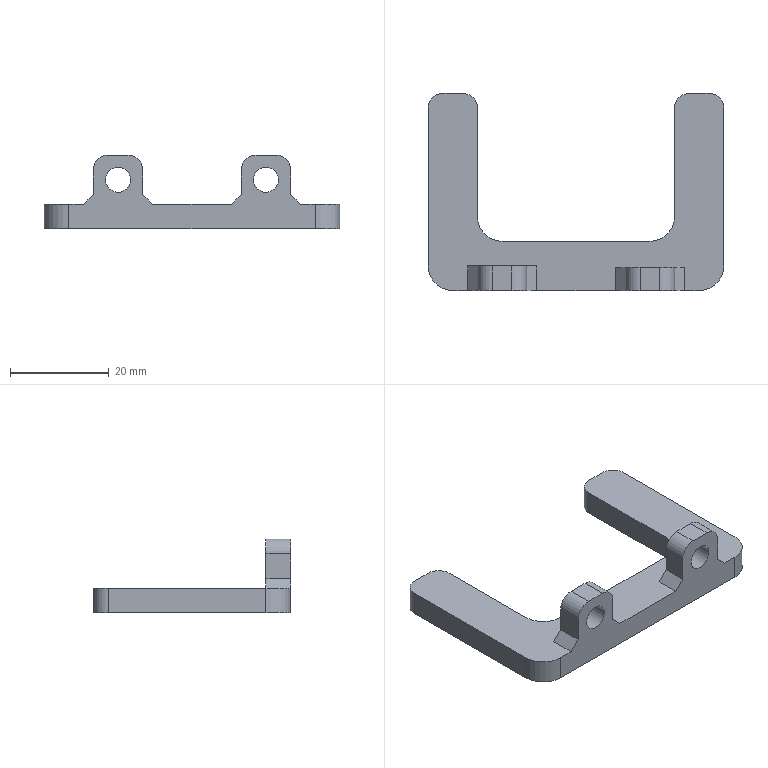Part | NX | features BREP 1 | 1 solid | 36 faces | box 60 x 40 x 15 mm | volume 6735 mm3 | plane 22 | cylinder 14 | commonest cylinder face diameters 6 x8 10 x4 5.1 x2
STEP:
#1=CARTESIAN_POINT('',(15.,-20.,7.45));
#2=VERTEX_POINT('',#1);
#3=CARTESIAN_POINT('',(15.,-20.,10.));
#4=DIRECTION('',(0.,-1.,0.));
#5=DIRECTION('',(0.,0.,-1.));
#6=AXIS2_PLACEMENT_3D('',#3,#4,#5);
#7=CIRCLE('',#6,2.55);
#8=EDGE_CURVE('',#2,#2,#7,.T.);
#9=ORIENTED_EDGE('',*,*,#8,.T.);
#10=EDGE_LOOP('',(#9));
#11=FACE_BOUND('',#10,.T.);
#12=CARTESIAN_POINT('',(15.,-15.3,7.45));
#13=VERTEX_POINT('',#12);
#14=CARTESIAN_POINT('',(15.,-15.3,10.));
#15=DIRECTION('',(0.,-1.,0.));
#16=DIRECTION('',(0.,0.,-1.));
#17=AXIS2_PLACEMENT_3D('',#14,#15,#16);
#18=CIRCLE('',#17,2.55);
#19=EDGE_CURVE('',#13,#13,#18,.T.);
#20=ORIENTED_EDGE('',*,*,#19,.F.);
#21=EDGE_LOOP('',(#20));
#22=FACE_BOUND('',#21,.T.);
#23=CARTESIAN_POINT('',(15.,-10.,10.));
#24=DIRECTION('',(0.,-1.,0.));
#25=DIRECTION('',(0.,0.,1.));
#26=AXIS2_PLACEMENT_3D('',#23,#24,#25);
#27=CYLINDRICAL_SURFACE('',#26,2.55);
#28=ADVANCED_FACE('',(#11,#22),#27,.F.);
#29=CARTESIAN_POINT('',(-15.,-20.,7.45));
#30=VERTEX_POINT('',#29);
#31=CARTESIAN_POINT('',(-15.,-20.,10.));
#32=DIRECTION('',(0.,-1.,0.));
#33=DIRECTION('',(0.,0.,-1.));
#34=AXIS2_PLACEMENT_3D('',#31,#32,#33);
#35=CIRCLE('',#34,2.55);
#36=EDGE_CURVE('',#30,#30,#35,.T.);
#37=ORIENTED_EDGE('',*,*,#36,.T.);
#38=EDGE_LOOP('',(#37));
#39=FACE_BOUND('',#38,.T.);
#40=CARTESIAN_POINT('',(-15.,-15.,7.45));
#41=VERTEX_POINT('',#40);
#42=CARTESIAN_POINT('',(-15.,-15.,10.));
#43=DIRECTION('',(0.,-1.,0.));
#44=DIRECTION('',(0.,0.,-1.));
#45=AXIS2_PLACEMENT_3D('',#42,#43,#44);
#46=CIRCLE('',#45,2.55);
#47=EDGE_CURVE('',#41,#41,#46,.T.);
#48=ORIENTED_EDGE('',*,*,#47,.F.);
#49=EDGE_LOOP('',(#48));
#50=FACE_BOUND('',#49,.T.);
#51=CARTESIAN_POINT('',(-15.,-10.,10.));
#52=DIRECTION('',(0.,-1.,0.));
#53=DIRECTION('',(0.,0.,1.));
#54=AXIS2_PLACEMENT_3D('',#51,#52,#53);
#55=CYLINDRICAL_SURFACE('',#54,2.55);
#56=ADVANCED_FACE('',(#39,#50),#55,.F.);
#57=CARTESIAN_POINT('',(22.,-15.3,5.));
#58=VERTEX_POINT('',#57);
#59=CARTESIAN_POINT('',(8.,-15.3,5.));
#60=VERTEX_POINT('',#59);
#61=CARTESIAN_POINT('',(10.,-15.3,5.));
#62=DIRECTION('',(-1.,0.,0.));
#63=VECTOR('',#62,1000.);
#64=LINE('',#61,#63);
#65=EDGE_CURVE('',#58,#60,#64,.T.);
#66=ORIENTED_EDGE('',*,*,#65,.F.);
#67=CARTESIAN_POINT('',(22.,-20.,5.));
#68=VERTEX_POINT('',#67);
#69=CARTESIAN_POINT('',(22.,0.,5.));
#70=DIRECTION('',(0.,-1.,0.));
#71=VECTOR('',#70,1000.);
#72=LINE('',#69,#71);
#73=EDGE_CURVE('',#58,#68,#72,.T.);
#74=ORIENTED_EDGE('',*,*,#73,.T.);
#75=CARTESIAN_POINT('',(25.,-20.,5.));
#76=VERTEX_POINT('',#75);
#77=CARTESIAN_POINT('',(-30.,-20.,5.));
#78=DIRECTION('',(1.,0.,0.));
#79=VECTOR('',#78,1000.);
#80=LINE('',#77,#79);
#81=EDGE_CURVE('',#68,#76,#80,.T.);
#82=ORIENTED_EDGE('',*,*,#81,.T.);
#83=CARTESIAN_POINT('',(30.,-15.,5.));
#84=VERTEX_POINT('',#83);
#85=CARTESIAN_POINT('',(25.,-15.,5.));
#86=DIRECTION('',(0.,0.,1.));
#87=DIRECTION('',(1.,0.,0.));
#88=AXIS2_PLACEMENT_3D('',#85,#86,#87);
#89=CIRCLE('',#88,5.);
#90=EDGE_CURVE('',#76,#84,#89,.T.);
#91=ORIENTED_EDGE('',*,*,#90,.T.);
#92=CARTESIAN_POINT('',(30.,17.,5.));
#93=VERTEX_POINT('',#92);
#94=CARTESIAN_POINT('',(30.,20.,5.));
#95=DIRECTION('',(0.,1.,0.));
#96=VECTOR('',#95,1000.);
#97=LINE('',#94,#96);
#98=EDGE_CURVE('',#84,#93,#97,.T.);
#99=ORIENTED_EDGE('',*,*,#98,.T.);
#100=CARTESIAN_POINT('',(27.,20.,5.));
#101=VERTEX_POINT('',#100);
#102=CARTESIAN_POINT('',(27.,17.,5.));
#103=DIRECTION('',(0.,0.,1.));
#104=DIRECTION('',(1.,0.,0.));
#105=AXIS2_PLACEMENT_3D('',#102,#103,#104);
#106=CIRCLE('',#105,3.);
#107=EDGE_CURVE('',#93,#101,#106,.T.);
#108=ORIENTED_EDGE('',*,*,#107,.T.);
#109=CARTESIAN_POINT('',(23.,20.,5.));
#110=VERTEX_POINT('',#109);
#111=CARTESIAN_POINT('',(-30.,20.,5.));
#112=DIRECTION('',(-1.,0.,0.));
#113=VECTOR('',#112,1000.);
#114=LINE('',#111,#113);
#115=EDGE_CURVE('',#101,#110,#114,.T.);
#116=ORIENTED_EDGE('',*,*,#115,.T.);
#117=CARTESIAN_POINT('',(20.,17.,5.));
#118=VERTEX_POINT('',#117);
#119=CARTESIAN_POINT('',(23.,17.,5.));
#120=DIRECTION('',(0.,0.,1.));
#121=DIRECTION('',(1.,0.,0.));
#122=AXIS2_PLACEMENT_3D('',#119,#120,#121);
#123=CIRCLE('',#122,3.);
#124=EDGE_CURVE('',#110,#118,#123,.T.);
#125=ORIENTED_EDGE('',*,*,#124,.T.);
#126=CARTESIAN_POINT('',(20.,-5.,5.));
#127=VERTEX_POINT('',#126);
#128=CARTESIAN_POINT('',(20.,20.,5.));
#129=DIRECTION('',(0.,1.,0.));
#130=VECTOR('',#129,1000.);
#131=LINE('',#128,#130);
#132=EDGE_CURVE('',#127,#118,#131,.T.);
#133=ORIENTED_EDGE('',*,*,#132,.F.);
#134=CARTESIAN_POINT('',(15.,-10.,5.));
#135=VERTEX_POINT('',#134);
#136=CARTESIAN_POINT('',(15.,-5.,5.));
#137=DIRECTION('',(0.,0.,-1.));
#138=DIRECTION('',(1.,0.,0.));
#139=AXIS2_PLACEMENT_3D('',#136,#137,#138);
#140=CIRCLE('',#139,5.);
#141=EDGE_CURVE('',#127,#135,#140,.T.);
#142=ORIENTED_EDGE('',*,*,#141,.T.);
#143=CARTESIAN_POINT('',(-15.,-10.,5.));
#144=VERTEX_POINT('',#143);
#145=CARTESIAN_POINT('',(-20.,-10.,5.));
#146=DIRECTION('',(1.,0.,0.));
#147=VECTOR('',#146,1000.);
#148=LINE('',#145,#147);
#149=EDGE_CURVE('',#144,#135,#148,.T.);
#150=ORIENTED_EDGE('',*,*,#149,.F.);
#151=CARTESIAN_POINT('',(-20.,-5.,5.));
#152=VERTEX_POINT('',#151);
#153=CARTESIAN_POINT('',(-15.,-5.,5.));
#154=DIRECTION('',(0.,0.,-1.));
#155=DIRECTION('',(1.,0.,0.));
#156=AXIS2_PLACEMENT_3D('',#153,#154,#155);
#157=CIRCLE('',#156,5.);
#158=EDGE_CURVE('',#144,#152,#157,.T.);
#159=ORIENTED_EDGE('',*,*,#158,.T.);
#160=CARTESIAN_POINT('',(-20.,17.,5.));
#161=VERTEX_POINT('',#160);
#162=CARTESIAN_POINT('',(-20.,20.,5.));
#163=DIRECTION('',(0.,-1.,0.));
#164=VECTOR('',#163,1000.);
#165=LINE('',#162,#164);
#166=EDGE_CURVE('',#161,#152,#165,.T.);
#167=ORIENTED_EDGE('',*,*,#166,.F.);
#168=CARTESIAN_POINT('',(-23.,20.,5.));
#169=VERTEX_POINT('',#168);
#170=CARTESIAN_POINT('',(-23.,17.,5.));
#171=DIRECTION('',(0.,0.,1.));
#172=DIRECTION('',(1.,0.,0.));
#173=AXIS2_PLACEMENT_3D('',#170,#171,#172);
#174=CIRCLE('',#173,3.);
#175=EDGE_CURVE('',#161,#169,#174,.T.);
#176=ORIENTED_EDGE('',*,*,#175,.T.);
#177=CARTESIAN_POINT('',(-27.,20.,5.));
#178=VERTEX_POINT('',#177);
#179=CARTESIAN_POINT('',(-30.,20.,5.));
#180=DIRECTION('',(-1.,0.,0.));
#181=VECTOR('',#180,1000.);
#182=LINE('',#179,#181);
#183=EDGE_CURVE('',#169,#178,#182,.T.);
#184=ORIENTED_EDGE('',*,*,#183,.T.);
#185=CARTESIAN_POINT('',(-30.,17.,5.));
#186=VERTEX_POINT('',#185);
#187=CARTESIAN_POINT('',(-27.,17.,5.));
#188=DIRECTION('',(0.,0.,1.));
#189=DIRECTION('',(1.,0.,0.));
#190=AXIS2_PLACEMENT_3D('',#187,#188,#189);
#191=CIRCLE('',#190,3.);
#192=EDGE_CURVE('',#178,#186,#191,.T.);
#193=ORIENTED_EDGE('',*,*,#192,.T.);
#194=CARTESIAN_POINT('',(-30.,-15.,5.));
#195=VERTEX_POINT('',#194);
#196=CARTESIAN_POINT('',(-30.,20.,5.));
#197=DIRECTION('',(0.,-1.,0.));
#198=VECTOR('',#197,1000.);
#199=LINE('',#196,#198);
#200=EDGE_CURVE('',#186,#195,#199,.T.);
#201=ORIENTED_EDGE('',*,*,#200,.T.);
#202=CARTESIAN_POINT('',(-25.,-20.,5.));
#203=VERTEX_POINT('',#202);
#204=CARTESIAN_POINT('',(-25.,-15.,5.));
#205=DIRECTION('',(0.,0.,1.));
#206=DIRECTION('',(1.,0.,0.));
#207=AXIS2_PLACEMENT_3D('',#204,#205,#206);
#208=CIRCLE('',#207,5.);
#209=EDGE_CURVE('',#195,#203,#208,.T.);
#210=ORIENTED_EDGE('',*,*,#209,.T.);
#211=CARTESIAN_POINT('',(-22.,-20.,5.));
#212=VERTEX_POINT('',#211);
#213=CARTESIAN_POINT('',(-30.,-20.,5.));
#214=DIRECTION('',(1.,0.,0.));
#215=VECTOR('',#214,1000.);
#216=LINE('',#213,#215);
#217=EDGE_CURVE('',#203,#212,#216,.T.);
#218=ORIENTED_EDGE('',*,*,#217,.T.);
#219=CARTESIAN_POINT('',(-22.,-15.,5.));
#220=VERTEX_POINT('',#219);
#221=CARTESIAN_POINT('',(-22.,0.,5.));
#222=DIRECTION('',(0.,1.,0.));
#223=VECTOR('',#222,1000.);
#224=LINE('',#221,#223);
#225=EDGE_CURVE('',#212,#220,#224,.T.);
#226=ORIENTED_EDGE('',*,*,#225,.T.);
#227=CARTESIAN_POINT('',(-8.,-15.,5.));
#228=VERTEX_POINT('',#227);
#229=CARTESIAN_POINT('',(-20.,-15.,5.));
#230=DIRECTION('',(-1.,0.,0.));
#231=VECTOR('',#230,1000.);
#232=LINE('',#229,#231);
#233=EDGE_CURVE('',#228,#220,#232,.T.);
#234=ORIENTED_EDGE('',*,*,#233,.F.);
#235=CARTESIAN_POINT('',(-8.,-20.,5.));
#236=VERTEX_POINT('',#235);
#237=CARTESIAN_POINT('',(-8.,0.,5.));
#238=DIRECTION('',(0.,-1.,0.));
#239=VECTOR('',#238,1000.);
#240=LINE('',#237,#239);
#241=EDGE_CURVE('',#228,#236,#240,.T.);
#242=ORIENTED_EDGE('',*,*,#241,.T.);
#243=CARTESIAN_POINT('',(8.,-20.,5.));
#244=VERTEX_POINT('',#243);
#245=CARTESIAN_POINT('',(-30.,-20.,5.));
#246=DIRECTION('',(1.,0.,0.));
#247=VECTOR('',#246,1000.);
#248=LINE('',#245,#247);
#249=EDGE_CURVE('',#236,#244,#248,.T.);
#250=ORIENTED_EDGE('',*,*,#249,.T.);
#251=CARTESIAN_POINT('',(8.,0.,5.));
#252=DIRECTION('',(0.,1.,0.));
#253=VECTOR('',#252,1000.);
#254=LINE('',#251,#253);
#255=EDGE_CURVE('',#244,#60,#254,.T.);
#256=ORIENTED_EDGE('',*,*,#255,.T.);
#257=EDGE_LOOP('',(#66,#74,#82,#91,#99,#108,#116,#125,#133,#142,#150,#159,#167,#176,#184,#193,#201,#210,#218,#226,#234,#242,#250,#256));
#258=FACE_BOUND('',#257,.T.);
#259=CARTESIAN_POINT('',(0.,0.,5.));
#260=DIRECTION('',(0.,0.,1.));
#261=DIRECTION('',(-1.,0.,0.));
#262=AXIS2_PLACEMENT_3D('',#259,#260,#261);
#263=PLANE('',#262);
#264=ADVANCED_FACE('',(#258),#263,.T.);
#265=CARTESIAN_POINT('',(-23.,20.,0.));
#266=VERTEX_POINT('',#265);
#267=CARTESIAN_POINT('',(-27.,20.,0.));
#268=VERTEX_POINT('',#267);
#269=CARTESIAN_POINT('',(-30.,20.,0.));
#270=DIRECTION('',(-1.,0.,0.));
#271=VECTOR('',#270,1000.);
#272=LINE('',#269,#271);
#273=EDGE_CURVE('',#266,#268,#272,.T.);
#274=ORIENTED_EDGE('',*,*,#273,.T.);
#275=CARTESIAN_POINT('',(-27.,20.,5.));
#276=DIRECTION('',(0.,0.,1.));
#277=VECTOR('',#276,1000.);
#278=LINE('',#275,#277);
#279=EDGE_CURVE('',#268,#178,#278,.T.);
#280=ORIENTED_EDGE('',*,*,#279,.T.);
#281=ORIENTED_EDGE('',*,*,#183,.F.);
#282=CARTESIAN_POINT('',(-23.,20.,5.));
#283=DIRECTION('',(0.,0.,-1.));
#284=VECTOR('',#283,1000.);
#285=LINE('',#282,#284);
#286=EDGE_CURVE('',#169,#266,#285,.T.);
#287=ORIENTED_EDGE('',*,*,#286,.T.);
#288=EDGE_LOOP('',(#274,#280,#281,#287));
#289=FACE_BOUND('',#288,.T.);
#290=CARTESIAN_POINT('',(-30.,20.,5.));
#291=DIRECTION('',(0.,-1.,0.));
#292=DIRECTION('',(0.,0.,1.));
#293=AXIS2_PLACEMENT_3D('',#290,#291,#292);
#294=PLANE('',#293);
#295=ADVANCED_FACE('',(#289),#294,.F.);
#296=CARTESIAN_POINT('',(30.,-15.,0.));
#297=VERTEX_POINT('',#296);
#298=CARTESIAN_POINT('',(30.,17.,0.));
#299=VERTEX_POINT('',#298);
#300=CARTESIAN_POINT('',(30.,20.,0.));
#301=DIRECTION('',(0.,1.,0.));
#302=VECTOR('',#301,1000.);
#303=LINE('',#300,#302);
#304=EDGE_CURVE('',#297,#299,#303,.T.);
#305=ORIENTED_EDGE('',*,*,#304,.T.);
#306=CARTESIAN_POINT('',(30.,17.,5.));
#307=DIRECTION('',(0.,0.,1.));
#308=VECTOR('',#307,1000.);
#309=LINE('',#306,#308);
#310=EDGE_CURVE('',#299,#93,#309,.T.);
#311=ORIENTED_EDGE('',*,*,#310,.T.);
#312=ORIENTED_EDGE('',*,*,#98,.F.);
#313=CARTESIAN_POINT('',(30.,-15.,5.));
#314=DIRECTION('',(0.,0.,-1.));
#315=VECTOR('',#314,1000.);
#316=LINE('',#313,#315);
#317=EDGE_CURVE('',#84,#297,#316,.T.);
#318=ORIENTED_EDGE('',*,*,#317,.T.);
#319=EDGE_LOOP('',(#305,#311,#312,#318));
#320=FACE_BOUND('',#319,.T.);
#321=CARTESIAN_POINT('',(30.,20.,5.));
#322=DIRECTION('',(-1.,0.,0.));
#323=DIRECTION('',(0.,1.,0.));
#324=AXIS2_PLACEMENT_3D('',#321,#322,#323);
#325=PLANE('',#324);
#326=ADVANCED_FACE('',(#320),#325,.F.);
#327=ORIENTED_EDGE('',*,*,#115,.F.);
#328=CARTESIAN_POINT('',(27.,20.,0.));
#329=VERTEX_POINT('',#328);
#330=CARTESIAN_POINT('',(27.,20.,5.));
#331=DIRECTION('',(0.,0.,-1.));
#332=VECTOR('',#331,1000.);
#333=LINE('',#330,#332);
#334=EDGE_CURVE('',#101,#329,#333,.T.);
#335=ORIENTED_EDGE('',*,*,#334,.T.);
#336=CARTESIAN_POINT('',(23.,20.,0.));
#337=VERTEX_POINT('',#336);
#338=CARTESIAN_POINT('',(-30.,20.,0.));
#339=DIRECTION('',(-1.,0.,0.));
#340=VECTOR('',#339,1000.);
#341=LINE('',#338,#340);
#342=EDGE_CURVE('',#329,#337,#341,.T.);
#343=ORIENTED_EDGE('',*,*,#342,.T.);
#344=CARTESIAN_POINT('',(23.,20.,5.));
#345=DIRECTION('',(0.,0.,1.));
#346=VECTOR('',#345,1000.);
#347=LINE('',#344,#346);
#348=EDGE_CURVE('',#337,#110,#347,.T.);
#349=ORIENTED_EDGE('',*,*,#348,.T.);
#350=EDGE_LOOP('',(#327,#335,#343,#349));
#351=FACE_BOUND('',#350,.T.);
#352=CARTESIAN_POINT('',(-30.,20.,5.));
#353=DIRECTION('',(0.,-1.,0.));
#354=DIRECTION('',(0.,0.,1.));
#355=AXIS2_PLACEMENT_3D('',#352,#353,#354);
#356=PLANE('',#355);
#357=ADVANCED_FACE('',(#351),#356,.F.);
#358=ORIENTED_EDGE('',*,*,#200,.F.);
#359=CARTESIAN_POINT('',(-30.,17.,0.));
#360=VERTEX_POINT('',#359);
#361=CARTESIAN_POINT('',(-30.,17.,5.));
#362=DIRECTION('',(0.,0.,-1.));
#363=VECTOR('',#362,1000.);
#364=LINE('',#361,#363);
#365=EDGE_CURVE('',#186,#360,#364,.T.);
#366=ORIENTED_EDGE('',*,*,#365,.T.);
#367=CARTESIAN_POINT('',(-30.,-15.,0.));
#368=VERTEX_POINT('',#367);
#369=CARTESIAN_POINT('',(-30.,20.,0.));
#370=DIRECTION('',(0.,-1.,0.));
#371=VECTOR('',#370,1000.);
#372=LINE('',#369,#371);
#373=EDGE_CURVE('',#360,#368,#372,.T.);
#374=ORIENTED_EDGE('',*,*,#373,.T.);
#375=CARTESIAN_POINT('',(-30.,-15.,5.));
#376=DIRECTION('',(0.,0.,1.));
#377=VECTOR('',#376,1000.);
#378=LINE('',#375,#377);
#379=EDGE_CURVE('',#368,#195,#378,.T.);
#380=ORIENTED_EDGE('',*,*,#379,.T.);
#381=EDGE_LOOP('',(#358,#366,#374,#380));
#382=FACE_BOUND('',#381,.T.);
#383=CARTESIAN_POINT('',(-30.,20.,5.));
#384=DIRECTION('',(1.,0.,0.));
#385=DIRECTION('',(0.,-1.,0.));
#386=AXIS2_PLACEMENT_3D('',#383,#384,#385);
#387=PLANE('',#386);
#388=ADVANCED_FACE('',(#382),#387,.F.);
#389=ORIENTED_EDGE('',*,*,#8,.F.);
#390=EDGE_LOOP('',(#389));
#391=FACE_BOUND('',#390,.T.);
#392=ORIENTED_EDGE('',*,*,#36,.F.);
#393=EDGE_LOOP('',(#392));
#394=FACE_BOUND('',#393,.T.);
#395=CARTESIAN_POINT('',(-17.,-20.,15.));
#396=VERTEX_POINT('',#395);
#397=CARTESIAN_POINT('',(-13.,-20.,15.));
#398=VERTEX_POINT('',#397);
#399=CARTESIAN_POINT('',(-20.,-20.,15.));
#400=DIRECTION('',(1.,0.,0.));
#401=VECTOR('',#400,1000.);
#402=LINE('',#399,#401);
#403=EDGE_CURVE('',#396,#398,#402,.T.);
#404=ORIENTED_EDGE('',*,*,#403,.F.);
#405=CARTESIAN_POINT('',(-20.,-20.,12.));
#406=VERTEX_POINT('',#405);
#407=CARTESIAN_POINT('',(-17.,-20.,12.));
#408=DIRECTION('',(0.,-1.,0.));
#409=DIRECTION('',(0.,0.,1.));
#410=AXIS2_PLACEMENT_3D('',#407,#408,#409);
#411=CIRCLE('',#410,3.);
#412=EDGE_CURVE('',#396,#406,#411,.T.);
#413=ORIENTED_EDGE('',*,*,#412,.T.);
#414=CARTESIAN_POINT('',(-20.,-20.,7.));
#415=VERTEX_POINT('',#414);
#416=CARTESIAN_POINT('',(-20.,-20.,15.));
#417=DIRECTION('',(0.,0.,-1.));
#418=VECTOR('',#417,1000.);
#419=LINE('',#416,#418);
#420=EDGE_CURVE('',#406,#415,#419,.T.);
#421=ORIENTED_EDGE('',*,*,#420,.T.);
#422=CARTESIAN_POINT('',(-26.,-20.,1.));
#423=DIRECTION('',(-0.7071,0.,-0.7071));
#424=VECTOR('',#423,1000.);
#425=LINE('',#422,#424);
#426=EDGE_CURVE('',#415,#212,#425,.T.);
#427=ORIENTED_EDGE('',*,*,#426,.T.);
#428=ORIENTED_EDGE('',*,*,#217,.F.);
#429=CARTESIAN_POINT('',(-25.,-20.,0.));
#430=VERTEX_POINT('',#429);
#431=CARTESIAN_POINT('',(-25.,-20.,5.));
#432=DIRECTION('',(0.,0.,-1.));
#433=VECTOR('',#432,1000.);
#434=LINE('',#431,#433);
#435=EDGE_CURVE('',#203,#430,#434,.T.);
#436=ORIENTED_EDGE('',*,*,#435,.T.);
#437=CARTESIAN_POINT('',(25.,-20.,0.));
#438=VERTEX_POINT('',#437);
#439=CARTESIAN_POINT('',(-30.,-20.,0.));
#440=DIRECTION('',(1.,0.,0.));
#441=VECTOR('',#440,1000.);
#442=LINE('',#439,#441);
#443=EDGE_CURVE('',#430,#438,#442,.T.);
#444=ORIENTED_EDGE('',*,*,#443,.T.);
#445=CARTESIAN_POINT('',(25.,-20.,5.));
#446=DIRECTION('',(0.,0.,1.));
#447=VECTOR('',#446,1000.);
#448=LINE('',#445,#447);
#449=EDGE_CURVE('',#438,#76,#448,.T.);
#450=ORIENTED_EDGE('',*,*,#449,.T.);
#451=ORIENTED_EDGE('',*,*,#81,.F.);
#452=CARTESIAN_POINT('',(20.,-20.,7.));
#453=VERTEX_POINT('',#452);
#454=CARTESIAN_POINT('',(-4.,-20.,31.));
#455=DIRECTION('',(-0.7071,0.,0.7071));
#456=VECTOR('',#455,1000.);
#457=LINE('',#454,#456);
#458=EDGE_CURVE('',#68,#453,#457,.T.);
#459=ORIENTED_EDGE('',*,*,#458,.T.);
#460=CARTESIAN_POINT('',(20.,-20.,12.));
#461=VERTEX_POINT('',#460);
#462=CARTESIAN_POINT('',(20.,-20.,15.));
#463=DIRECTION('',(0.,0.,-1.));
#464=VECTOR('',#463,1000.);
#465=LINE('',#462,#464);
#466=EDGE_CURVE('',#461,#453,#465,.T.);
#467=ORIENTED_EDGE('',*,*,#466,.F.);
#468=CARTESIAN_POINT('',(17.,-20.,15.));
#469=VERTEX_POINT('',#468);
#470=CARTESIAN_POINT('',(17.,-20.,12.));
#471=DIRECTION('',(0.,-1.,0.));
#472=DIRECTION('',(0.,0.,1.));
#473=AXIS2_PLACEMENT_3D('',#470,#471,#472);
#474=CIRCLE('',#473,3.);
#475=EDGE_CURVE('',#461,#469,#474,.T.);
#476=ORIENTED_EDGE('',*,*,#475,.T.);
#477=CARTESIAN_POINT('',(13.,-20.,15.));
#478=VERTEX_POINT('',#477);
#479=CARTESIAN_POINT('',(10.,-20.,15.));
#480=DIRECTION('',(1.,0.,0.));
#481=VECTOR('',#480,1000.);
#482=LINE('',#479,#481);
#483=EDGE_CURVE('',#478,#469,#482,.T.);
#484=ORIENTED_EDGE('',*,*,#483,.F.);
#485=CARTESIAN_POINT('',(10.,-20.,12.));
#486=VERTEX_POINT('',#485);
#487=CARTESIAN_POINT('',(13.,-20.,12.));
#488=DIRECTION('',(0.,-1.,0.));
#489=DIRECTION('',(0.,0.,1.));
#490=AXIS2_PLACEMENT_3D('',#487,#488,#489);
#491=CIRCLE('',#490,3.);
#492=EDGE_CURVE('',#478,#486,#491,.T.);
#493=ORIENTED_EDGE('',*,*,#492,.T.);
#494=CARTESIAN_POINT('',(10.,-20.,7.));
#495=VERTEX_POINT('',#494);
#496=CARTESIAN_POINT('',(10.,-20.,15.));
#497=DIRECTION('',(0.,0.,-1.));
#498=VECTOR('',#497,1000.);
#499=LINE('',#496,#498);
#500=EDGE_CURVE('',#486,#495,#499,.T.);
#501=ORIENTED_EDGE('',*,*,#500,.T.);
#502=CARTESIAN_POINT('',(-11.,-20.,-14.));
#503=DIRECTION('',(-0.7071,0.,-0.7071));
#504=VECTOR('',#503,1000.);
#505=LINE('',#502,#504);
#506=EDGE_CURVE('',#495,#244,#505,.T.);
#507=ORIENTED_EDGE('',*,*,#506,.T.);
#508=ORIENTED_EDGE('',*,*,#249,.F.);
#509=CARTESIAN_POINT('',(-10.,-20.,7.));
#510=VERTEX_POINT('',#509);
#511=CARTESIAN_POINT('',(-19.,-20.,16.));
#512=DIRECTION('',(-0.7071,0.,0.7071));
#513=VECTOR('',#512,1000.);
#514=LINE('',#511,#513);
#515=EDGE_CURVE('',#236,#510,#514,.T.);
#516=ORIENTED_EDGE('',*,*,#515,.T.);
#517=CARTESIAN_POINT('',(-10.,-20.,12.));
#518=VERTEX_POINT('',#517);
#519=CARTESIAN_POINT('',(-10.,-20.,15.));
#520=DIRECTION('',(0.,0.,-1.));
#521=VECTOR('',#520,1000.);
#522=LINE('',#519,#521);
#523=EDGE_CURVE('',#518,#510,#522,.T.);
#524=ORIENTED_EDGE('',*,*,#523,.F.);
#525=CARTESIAN_POINT('',(-13.,-20.,12.));
#526=DIRECTION('',(0.,-1.,0.));
#527=DIRECTION('',(0.,0.,1.));
#528=AXIS2_PLACEMENT_3D('',#525,#526,#527);
#529=CIRCLE('',#528,3.);
#530=EDGE_CURVE('',#518,#398,#529,.T.);
#531=ORIENTED_EDGE('',*,*,#530,.T.);
#532=EDGE_LOOP('',(#404,#413,#421,#427,#428,#436,#444,#450,#451,#459,#467,#476,#484,#493,#501,#507,#508,#516,#524,#531));
#533=FACE_BOUND('',#532,.T.);
#534=CARTESIAN_POINT('',(-30.,-20.,5.));
#535=DIRECTION('',(0.,1.,0.));
#536=DIRECTION('',(0.,0.,-1.));
#537=AXIS2_PLACEMENT_3D('',#534,#535,#536);
#538=PLANE('',#537);
#539=ADVANCED_FACE('',(#391,#394,#533),#538,.F.);
#540=ORIENTED_EDGE('',*,*,#342,.F.);
#541=CARTESIAN_POINT('',(27.,17.,0.));
#542=DIRECTION('',(0.,0.,-1.));
#543=DIRECTION('',(1.,0.,0.));
#544=AXIS2_PLACEMENT_3D('',#541,#542,#543);
#545=CIRCLE('',#544,3.);
#546=EDGE_CURVE('',#329,#299,#545,.T.);
#547=ORIENTED_EDGE('',*,*,#546,.T.);
#548=ORIENTED_EDGE('',*,*,#304,.F.);
#549=CARTESIAN_POINT('',(25.,-15.,0.));
#550=DIRECTION('',(0.,0.,-1.));
#551=DIRECTION('',(1.,0.,0.));
#552=AXIS2_PLACEMENT_3D('',#549,#550,#551);
#553=CIRCLE('',#552,5.);
#554=EDGE_CURVE('',#297,#438,#553,.T.);
#555=ORIENTED_EDGE('',*,*,#554,.T.);
#556=ORIENTED_EDGE('',*,*,#443,.F.);
#557=CARTESIAN_POINT('',(-25.,-15.,0.));
#558=DIRECTION('',(0.,0.,-1.));
#559=DIRECTION('',(1.,0.,0.));
#560=AXIS2_PLACEMENT_3D('',#557,#558,#559);
#561=CIRCLE('',#560,5.);
#562=EDGE_CURVE('',#430,#368,#561,.T.);
#563=ORIENTED_EDGE('',*,*,#562,.T.);
#564=ORIENTED_EDGE('',*,*,#373,.F.);
#565=CARTESIAN_POINT('',(-27.,17.,0.));
#566=DIRECTION('',(0.,0.,-1.));
#567=DIRECTION('',(1.,0.,0.));
#568=AXIS2_PLACEMENT_3D('',#565,#566,#567);
#569=CIRCLE('',#568,3.);
#570=EDGE_CURVE('',#360,#268,#569,.T.);
#571=ORIENTED_EDGE('',*,*,#570,.T.);
#572=ORIENTED_EDGE('',*,*,#273,.F.);
#573=CARTESIAN_POINT('',(-20.,17.,0.));
#574=VERTEX_POINT('',#573);
#575=CARTESIAN_POINT('',(-23.,17.,0.));
#576=DIRECTION('',(0.,0.,-1.));
#577=DIRECTION('',(1.,0.,0.));
#578=AXIS2_PLACEMENT_3D('',#575,#576,#577);
#579=CIRCLE('',#578,3.);
#580=EDGE_CURVE('',#266,#574,#579,.T.);
#581=ORIENTED_EDGE('',*,*,#580,.T.);
#582=CARTESIAN_POINT('',(-20.,-5.,0.));
#583=VERTEX_POINT('',#582);
#584=CARTESIAN_POINT('',(-20.,20.,0.));
#585=DIRECTION('',(0.,-1.,0.));
#586=VECTOR('',#585,1000.);
#587=LINE('',#584,#586);
#588=EDGE_CURVE('',#574,#583,#587,.T.);
#589=ORIENTED_EDGE('',*,*,#588,.T.);
#590=CARTESIAN_POINT('',(-15.,-10.,0.));
#591=VERTEX_POINT('',#590);
#592=CARTESIAN_POINT('',(-15.,-5.,0.));
#593=DIRECTION('',(0.,0.,1.));
#594=DIRECTION('',(1.,0.,0.));
#595=AXIS2_PLACEMENT_3D('',#592,#593,#594);
#596=CIRCLE('',#595,5.);
#597=EDGE_CURVE('',#583,#591,#596,.T.);
#598=ORIENTED_EDGE('',*,*,#597,.T.);
#599=CARTESIAN_POINT('',(15.,-10.,0.));
#600=VERTEX_POINT('',#599);
#601=CARTESIAN_POINT('',(-20.,-10.,0.));
#602=DIRECTION('',(1.,0.,0.));
#603=VECTOR('',#602,1000.);
#604=LINE('',#601,#603);
#605=EDGE_CURVE('',#591,#600,#604,.T.);
#606=ORIENTED_EDGE('',*,*,#605,.T.);
#607=CARTESIAN_POINT('',(20.,-5.,0.));
#608=VERTEX_POINT('',#607);
#609=CARTESIAN_POINT('',(15.,-5.,0.));
#610=DIRECTION('',(0.,0.,1.));
#611=DIRECTION('',(1.,0.,0.));
#612=AXIS2_PLACEMENT_3D('',#609,#610,#611);
#613=CIRCLE('',#612,5.);
#614=EDGE_CURVE('',#600,#608,#613,.T.);
#615=ORIENTED_EDGE('',*,*,#614,.T.);
#616=CARTESIAN_POINT('',(20.,17.,0.));
#617=VERTEX_POINT('',#616);
#618=CARTESIAN_POINT('',(20.,20.,0.));
#619=DIRECTION('',(0.,1.,0.));
#620=VECTOR('',#619,1000.);
#621=LINE('',#618,#620);
#622=EDGE_CURVE('',#608,#617,#621,.T.);
#623=ORIENTED_EDGE('',*,*,#622,.T.);
#624=CARTESIAN_POINT('',(23.,17.,0.));
#625=DIRECTION('',(0.,0.,-1.));
#626=DIRECTION('',(1.,0.,0.));
#627=AXIS2_PLACEMENT_3D('',#624,#625,#626);
#628=CIRCLE('',#627,3.);
#629=EDGE_CURVE('',#617,#337,#628,.T.);
#630=ORIENTED_EDGE('',*,*,#629,.T.);
#631=EDGE_LOOP('',(#540,#547,#548,#555,#556,#563,#564,#571,#572,#581,#589,#598,#606,#615,#623,#630));
#632=FACE_BOUND('',#631,.T.);
#633=CARTESIAN_POINT('',(0.,0.,0.));
#634=DIRECTION('',(0.,0.,1.));
#635=DIRECTION('',(-1.,0.,0.));
#636=AXIS2_PLACEMENT_3D('',#633,#634,#635);
#637=PLANE('',#636);
#638=ADVANCED_FACE('',(#632),#637,.F.);
#639=ORIENTED_EDGE('',*,*,#588,.F.);
#640=CARTESIAN_POINT('',(-20.,17.,0.));
#641=DIRECTION('',(0.,0.,1.));
#642=VECTOR('',#641,1000.);
#643=LINE('',#640,#642);
#644=EDGE_CURVE('',#574,#161,#643,.T.);
#645=ORIENTED_EDGE('',*,*,#644,.T.);
#646=ORIENTED_EDGE('',*,*,#166,.T.);
#647=CARTESIAN_POINT('',(-20.,-5.,0.));
#648=DIRECTION('',(0.,0.,-1.));
#649=VECTOR('',#648,1000.);
#650=LINE('',#647,#649);
#651=EDGE_CURVE('',#152,#583,#650,.T.);
#652=ORIENTED_EDGE('',*,*,#651,.T.);
#653=EDGE_LOOP('',(#639,#645,#646,#652));
#654=FACE_BOUND('',#653,.T.);
#655=CARTESIAN_POINT('',(-20.,20.,0.));
#656=DIRECTION('',(-1.,0.,0.));
#657=DIRECTION('',(0.,1.,0.));
#658=AXIS2_PLACEMENT_3D('',#655,#656,#657);
#659=PLANE('',#658);
#660=ADVANCED_FACE('',(#654),#659,.F.);
#661=ORIENTED_EDGE('',*,*,#132,.T.);
#662=CARTESIAN_POINT('',(20.,17.,0.));
#663=DIRECTION('',(0.,0.,-1.));
#664=VECTOR('',#663,1000.);
#665=LINE('',#662,#664);
#666=EDGE_CURVE('',#118,#617,#665,.T.);
#667=ORIENTED_EDGE('',*,*,#666,.T.);
#668=ORIENTED_EDGE('',*,*,#622,.F.);
#669=CARTESIAN_POINT('',(20.,-5.,5.));
#670=DIRECTION('',(0.,0.,1.));
#671=VECTOR('',#670,1000.);
#672=LINE('',#669,#671);
#673=EDGE_CURVE('',#608,#127,#672,.T.);
#674=ORIENTED_EDGE('',*,*,#673,.T.);
#675=EDGE_LOOP('',(#661,#667,#668,#674));
#676=FACE_BOUND('',#675,.T.);
#677=CARTESIAN_POINT('',(20.,20.,0.));
#678=DIRECTION('',(1.,0.,0.));
#679=DIRECTION('',(0.,-1.,0.));
#680=AXIS2_PLACEMENT_3D('',#677,#678,#679);
#681=PLANE('',#680);
#682=ADVANCED_FACE('',(#676),#681,.F.);
#683=ORIENTED_EDGE('',*,*,#149,.T.);
#684=CARTESIAN_POINT('',(15.,-10.,0.));
#685=DIRECTION('',(0.,0.,-1.));
#686=VECTOR('',#685,1000.);
#687=LINE('',#684,#686);
#688=EDGE_CURVE('',#135,#600,#687,.T.);
#689=ORIENTED_EDGE('',*,*,#688,.T.);
#690=ORIENTED_EDGE('',*,*,#605,.F.);
#691=CARTESIAN_POINT('',(-15.,-10.,5.));
#692=DIRECTION('',(0.,0.,1.));
#693=VECTOR('',#692,1000.);
#694=LINE('',#691,#693);
#695=EDGE_CURVE('',#591,#144,#694,.T.);
#696=ORIENTED_EDGE('',*,*,#695,.T.);
#697=EDGE_LOOP('',(#683,#689,#690,#696));
#698=FACE_BOUND('',#697,.T.);
#699=CARTESIAN_POINT('',(-20.,-10.,0.));
#700=DIRECTION('',(0.,-1.,0.));
#701=DIRECTION('',(0.,0.,1.));
#702=AXIS2_PLACEMENT_3D('',#699,#700,#701);
#703=PLANE('',#702);
#704=ADVANCED_FACE('',(#698),#703,.F.);
#705=CARTESIAN_POINT('',(-20.,-15.,12.));
#706=VERTEX_POINT('',#705);
#707=CARTESIAN_POINT('',(-20.,-15.,7.));
#708=VERTEX_POINT('',#707);
#709=CARTESIAN_POINT('',(-20.,-15.,15.));
#710=DIRECTION('',(0.,0.,-1.));
#711=VECTOR('',#710,1000.);
#712=LINE('',#709,#711);
#713=EDGE_CURVE('',#706,#708,#712,.T.);
#714=ORIENTED_EDGE('',*,*,#713,.T.);
#715=CARTESIAN_POINT('',(-20.,-20.,7.));
#716=DIRECTION('',(0.,-1.,0.));
#717=VECTOR('',#716,1000.);
#718=LINE('',#715,#717);
#719=EDGE_CURVE('',#708,#415,#718,.T.);
#720=ORIENTED_EDGE('',*,*,#719,.T.);
#721=ORIENTED_EDGE('',*,*,#420,.F.);
#722=CARTESIAN_POINT('',(-20.,-20.,12.));
#723=DIRECTION('',(0.,1.,0.));
#724=VECTOR('',#723,1000.);
#725=LINE('',#722,#724);
#726=EDGE_CURVE('',#406,#706,#725,.T.);
#727=ORIENTED_EDGE('',*,*,#726,.T.);
#728=EDGE_LOOP('',(#714,#720,#721,#727));
#729=FACE_BOUND('',#728,.T.);
#730=CARTESIAN_POINT('',(-20.,-20.,15.));
#731=DIRECTION('',(1.,0.,0.));
#732=DIRECTION('',(0.,0.,1.));
#733=AXIS2_PLACEMENT_3D('',#730,#731,#732);
#734=PLANE('',#733);
#735=ADVANCED_FACE('',(#729),#734,.F.);
#736=ORIENTED_EDGE('',*,*,#523,.T.);
#737=CARTESIAN_POINT('',(-10.,-15.,7.));
#738=VERTEX_POINT('',#737);
#739=CARTESIAN_POINT('',(-10.,-20.,7.));
#740=DIRECTION('',(0.,1.,0.));
#741=VECTOR('',#740,1000.);
#742=LINE('',#739,#741);
#743=EDGE_CURVE('',#510,#738,#742,.T.);
#744=ORIENTED_EDGE('',*,*,#743,.T.);
#745=CARTESIAN_POINT('',(-10.,-15.,12.));
#746=VERTEX_POINT('',#745);
#747=CARTESIAN_POINT('',(-10.,-15.,15.));
#748=DIRECTION('',(0.,0.,-1.));
#749=VECTOR('',#748,1000.);
#750=LINE('',#747,#749);
#751=EDGE_CURVE('',#746,#738,#750,.T.);
#752=ORIENTED_EDGE('',*,*,#751,.F.);
#753=CARTESIAN_POINT('',(-10.,-20.,12.));
#754=DIRECTION('',(0.,-1.,0.));
#755=VECTOR('',#754,1000.);
#756=LINE('',#753,#755);
#757=EDGE_CURVE('',#746,#518,#756,.T.);
#758=ORIENTED_EDGE('',*,*,#757,.T.);
#759=EDGE_LOOP('',(#736,#744,#752,#758));
#760=FACE_BOUND('',#759,.T.);
#761=CARTESIAN_POINT('',(-10.,-20.,15.));
#762=DIRECTION('',(-1.,0.,0.));
#763=DIRECTION('',(0.,0.,-1.));
#764=AXIS2_PLACEMENT_3D('',#761,#762,#763);
#765=PLANE('',#764);
#766=ADVANCED_FACE('',(#760),#765,.F.);
#767=ORIENTED_EDGE('',*,*,#47,.T.);
#768=EDGE_LOOP('',(#767));
#769=FACE_BOUND('',#768,.T.);
#770=ORIENTED_EDGE('',*,*,#713,.F.);
#771=CARTESIAN_POINT('',(-17.,-15.,15.));
#772=VERTEX_POINT('',#771);
#773=CARTESIAN_POINT('',(-17.,-15.,12.));
#774=DIRECTION('',(0.,1.,0.));
#775=DIRECTION('',(0.,0.,-1.));
#776=AXIS2_PLACEMENT_3D('',#773,#774,#775);
#777=CIRCLE('',#776,3.);
#778=EDGE_CURVE('',#706,#772,#777,.T.);
#779=ORIENTED_EDGE('',*,*,#778,.T.);
#780=CARTESIAN_POINT('',(-13.,-15.,15.));
#781=VERTEX_POINT('',#780);
#782=CARTESIAN_POINT('',(-20.,-15.,15.));
#783=DIRECTION('',(-1.,0.,0.));
#784=VECTOR('',#783,1000.);
#785=LINE('',#782,#784);
#786=EDGE_CURVE('',#781,#772,#785,.T.);
#787=ORIENTED_EDGE('',*,*,#786,.F.);
#788=CARTESIAN_POINT('',(-13.,-15.,12.));
#789=DIRECTION('',(0.,1.,0.));
#790=DIRECTION('',(0.,0.,-1.));
#791=AXIS2_PLACEMENT_3D('',#788,#789,#790);
#792=CIRCLE('',#791,3.);
#793=EDGE_CURVE('',#781,#746,#792,.T.);
#794=ORIENTED_EDGE('',*,*,#793,.T.);
#795=ORIENTED_EDGE('',*,*,#751,.T.);
#796=CARTESIAN_POINT('',(-19.,-15.,16.));
#797=DIRECTION('',(0.7071,0.,-0.7071));
#798=VECTOR('',#797,1000.);
#799=LINE('',#796,#798);
#800=EDGE_CURVE('',#738,#228,#799,.T.);
#801=ORIENTED_EDGE('',*,*,#800,.T.);
#802=ORIENTED_EDGE('',*,*,#233,.T.);
#803=CARTESIAN_POINT('',(-16.,-15.,11.));
#804=DIRECTION('',(0.7071,0.,0.7071));
#805=VECTOR('',#804,1000.);
#806=LINE('',#803,#805);
#807=EDGE_CURVE('',#220,#708,#806,.T.);
#808=ORIENTED_EDGE('',*,*,#807,.T.);
#809=EDGE_LOOP('',(#770,#779,#787,#794,#795,#801,#802,#808));
#810=FACE_BOUND('',#809,.T.);
#811=CARTESIAN_POINT('',(-20.,-15.,15.));
#812=DIRECTION('',(0.,-1.,0.));
#813=DIRECTION('',(0.,0.,1.));
#814=AXIS2_PLACEMENT_3D('',#811,#812,#813);
#815=PLANE('',#814);
#816=ADVANCED_FACE('',(#769,#810),#815,.F.);
#817=ORIENTED_EDGE('',*,*,#786,.T.);
#818=CARTESIAN_POINT('',(-17.,0.,15.));
#819=DIRECTION('',(0.,-1.,0.));
#820=VECTOR('',#819,1000.);
#821=LINE('',#818,#820);
#822=EDGE_CURVE('',#772,#396,#821,.T.);
#823=ORIENTED_EDGE('',*,*,#822,.T.);
#824=ORIENTED_EDGE('',*,*,#403,.T.);
#825=CARTESIAN_POINT('',(-13.,0.,15.));
#826=DIRECTION('',(0.,1.,0.));
#827=VECTOR('',#826,1000.);
#828=LINE('',#825,#827);
#829=EDGE_CURVE('',#398,#781,#828,.T.);
#830=ORIENTED_EDGE('',*,*,#829,.T.);
#831=EDGE_LOOP('',(#817,#823,#824,#830));
#832=FACE_BOUND('',#831,.T.);
#833=CARTESIAN_POINT('',(0.,0.,15.));
#834=DIRECTION('',(0.,0.,-1.));
#835=DIRECTION('',(1.,0.,0.));
#836=AXIS2_PLACEMENT_3D('',#833,#834,#835);
#837=PLANE('',#836);
#838=ADVANCED_FACE('',(#832),#837,.F.);
#839=CARTESIAN_POINT('',(10.,-15.3,12.));
#840=VERTEX_POINT('',#839);
#841=CARTESIAN_POINT('',(10.,-15.3,7.));
#842=VERTEX_POINT('',#841);
#843=CARTESIAN_POINT('',(10.,-15.3,15.));
#844=DIRECTION('',(0.,0.,-1.));
#845=VECTOR('',#844,1000.);
#846=LINE('',#843,#845);
#847=EDGE_CURVE('',#840,#842,#846,.T.);
#848=ORIENTED_EDGE('',*,*,#847,.T.);
#849=CARTESIAN_POINT('',(10.,-20.,7.));
#850=DIRECTION('',(0.,-1.,0.));
#851=VECTOR('',#850,1000.);
#852=LINE('',#849,#851);
#853=EDGE_CURVE('',#842,#495,#852,.T.);
#854=ORIENTED_EDGE('',*,*,#853,.T.);
#855=ORIENTED_EDGE('',*,*,#500,.F.);
#856=CARTESIAN_POINT('',(10.,-20.,12.));
#857=DIRECTION('',(0.,1.,0.));
#858=VECTOR('',#857,1000.);
#859=LINE('',#856,#858);
#860=EDGE_CURVE('',#486,#840,#859,.T.);
#861=ORIENTED_EDGE('',*,*,#860,.T.);
#862=EDGE_LOOP('',(#848,#854,#855,#861));
#863=FACE_BOUND('',#862,.T.);
#864=CARTESIAN_POINT('',(10.,-20.,15.));
#865=DIRECTION('',(1.,0.,0.));
#866=DIRECTION('',(0.,-1.,0.));
#867=AXIS2_PLACEMENT_3D('',#864,#865,#866);
#868=PLANE('',#867);
#869=ADVANCED_FACE('',(#863),#868,.F.);
#870=ORIENTED_EDGE('',*,*,#466,.T.);
#871=CARTESIAN_POINT('',(20.,-15.3,7.));
#872=VERTEX_POINT('',#871);
#873=CARTESIAN_POINT('',(20.,-20.,7.));
#874=DIRECTION('',(0.,1.,0.));
#875=VECTOR('',#874,1000.);
#876=LINE('',#873,#875);
#877=EDGE_CURVE('',#453,#872,#876,.T.);
#878=ORIENTED_EDGE('',*,*,#877,.T.);
#879=CARTESIAN_POINT('',(20.,-15.3,12.));
#880=VERTEX_POINT('',#879);
#881=CARTESIAN_POINT('',(20.,-15.3,15.));
#882=DIRECTION('',(0.,0.,-1.));
#883=VECTOR('',#882,1000.);
#884=LINE('',#881,#883);
#885=EDGE_CURVE('',#880,#872,#884,.T.);
#886=ORIENTED_EDGE('',*,*,#885,.F.);
#887=CARTESIAN_POINT('',(20.,-20.,12.));
#888=DIRECTION('',(0.,-1.,0.));
#889=VECTOR('',#888,1000.);
#890=LINE('',#887,#889);
#891=EDGE_CURVE('',#880,#461,#890,.T.);
#892=ORIENTED_EDGE('',*,*,#891,.T.);
#893=EDGE_LOOP('',(#870,#878,#886,#892));
#894=FACE_BOUND('',#893,.T.);
#895=CARTESIAN_POINT('',(20.,-20.,15.));
#896=DIRECTION('',(-1.,0.,0.));
#897=DIRECTION('',(0.,0.,-1.));
#898=AXIS2_PLACEMENT_3D('',#895,#896,#897);
#899=PLANE('',#898);
#900=ADVANCED_FACE('',(#894),#899,.F.);
#901=ORIENTED_EDGE('',*,*,#19,.T.);
#902=EDGE_LOOP('',(#901));
#903=FACE_BOUND('',#902,.T.);
#904=ORIENTED_EDGE('',*,*,#847,.F.);
#905=CARTESIAN_POINT('',(13.,-15.3,15.));
#906=VERTEX_POINT('',#905);
#907=CARTESIAN_POINT('',(13.,-15.3,12.));
#908=DIRECTION('',(0.,1.,0.));
#909=DIRECTION('',(0.,0.,-1.));
#910=AXIS2_PLACEMENT_3D('',#907,#908,#909);
#911=CIRCLE('',#910,3.);
#912=EDGE_CURVE('',#840,#906,#911,.T.);
#913=ORIENTED_EDGE('',*,*,#912,.T.);
#914=CARTESIAN_POINT('',(17.,-15.3,15.));
#915=VERTEX_POINT('',#914);
#916=CARTESIAN_POINT('',(10.,-15.3,15.));
#917=DIRECTION('',(-1.,0.,0.));
#918=VECTOR('',#917,1000.);
#919=LINE('',#916,#918);
#920=EDGE_CURVE('',#915,#906,#919,.T.);
#921=ORIENTED_EDGE('',*,*,#920,.F.);
#922=CARTESIAN_POINT('',(17.,-15.3,12.));
#923=DIRECTION('',(0.,1.,0.));
#924=DIRECTION('',(0.,0.,-1.));
#925=AXIS2_PLACEMENT_3D('',#922,#923,#924);
#926=CIRCLE('',#925,3.);
#927=EDGE_CURVE('',#915,#880,#926,.T.);
#928=ORIENTED_EDGE('',*,*,#927,.T.);
#929=ORIENTED_EDGE('',*,*,#885,.T.);
#930=CARTESIAN_POINT('',(11.,-15.3,16.));
#931=DIRECTION('',(0.7071,0.,-0.7071));
#932=VECTOR('',#931,1000.);
#933=LINE('',#930,#932);
#934=EDGE_CURVE('',#872,#58,#933,.T.);
#935=ORIENTED_EDGE('',*,*,#934,.T.);
#936=ORIENTED_EDGE('',*,*,#65,.T.);
#937=CARTESIAN_POINT('',(14.,-15.3,11.));
#938=DIRECTION('',(0.7071,0.,0.7071));
#939=VECTOR('',#938,1000.);
#940=LINE('',#937,#939);
#941=EDGE_CURVE('',#60,#842,#940,.T.);
#942=ORIENTED_EDGE('',*,*,#941,.T.);
#943=EDGE_LOOP('',(#904,#913,#921,#928,#929,#935,#936,#942));
#944=FACE_BOUND('',#943,.T.);
#945=CARTESIAN_POINT('',(10.,-15.3,15.));
#946=DIRECTION('',(0.,-1.,0.));
#947=DIRECTION('',(0.,0.,1.));
#948=AXIS2_PLACEMENT_3D('',#945,#946,#947);
#949=PLANE('',#948);
#950=ADVANCED_FACE('',(#903,#944),#949,.F.);
#951=ORIENTED_EDGE('',*,*,#920,.T.);
#952=CARTESIAN_POINT('',(13.,0.,15.));
#953=DIRECTION('',(0.,-1.,0.));
#954=VECTOR('',#953,1000.);
#955=LINE('',#952,#954);
#956=EDGE_CURVE('',#906,#478,#955,.T.);
#957=ORIENTED_EDGE('',*,*,#956,.T.);
#958=ORIENTED_EDGE('',*,*,#483,.T.);
#959=CARTESIAN_POINT('',(17.,0.,15.));
#960=DIRECTION('',(0.,1.,0.));
#961=VECTOR('',#960,1000.);
#962=LINE('',#959,#961);
#963=EDGE_CURVE('',#469,#915,#962,.T.);
#964=ORIENTED_EDGE('',*,*,#963,.T.);
#965=EDGE_LOOP('',(#951,#957,#958,#964));
#966=FACE_BOUND('',#965,.T.);
#967=CARTESIAN_POINT('',(0.,0.,15.));
#968=DIRECTION('',(0.,0.,-1.));
#969=DIRECTION('',(1.,0.,0.));
#970=AXIS2_PLACEMENT_3D('',#967,#968,#969);
#971=PLANE('',#970);
#972=ADVANCED_FACE('',(#966),#971,.F.);
#973=ORIENTED_EDGE('',*,*,#90,.F.);
#974=ORIENTED_EDGE('',*,*,#449,.F.);
#975=ORIENTED_EDGE('',*,*,#554,.F.);
#976=ORIENTED_EDGE('',*,*,#317,.F.);
#977=EDGE_LOOP('',(#973,#974,#975,#976));
#978=FACE_BOUND('',#977,.T.);
#979=CARTESIAN_POINT('',(25.,-15.,5.));
#980=DIRECTION('',(0.,0.,-1.));
#981=DIRECTION('',(1.,0.,0.));
#982=AXIS2_PLACEMENT_3D('',#979,#980,#981);
#983=CYLINDRICAL_SURFACE('',#982,5.);
#984=ADVANCED_FACE('',(#978),#983,.T.);
#985=ORIENTED_EDGE('',*,*,#209,.F.);
#986=ORIENTED_EDGE('',*,*,#379,.F.);
#987=ORIENTED_EDGE('',*,*,#562,.F.);
#988=ORIENTED_EDGE('',*,*,#435,.F.);
#989=EDGE_LOOP('',(#985,#986,#987,#988));
#990=FACE_BOUND('',#989,.T.);
#991=CARTESIAN_POINT('',(-25.,-15.,5.));
#992=DIRECTION('',(0.,0.,-1.));
#993=DIRECTION('',(1.,0.,0.));
#994=AXIS2_PLACEMENT_3D('',#991,#992,#993);
#995=CYLINDRICAL_SURFACE('',#994,5.);
#996=ADVANCED_FACE('',(#990),#995,.T.);
#997=ORIENTED_EDGE('',*,*,#614,.F.);
#998=ORIENTED_EDGE('',*,*,#688,.F.);
#999=ORIENTED_EDGE('',*,*,#141,.F.);
#1000=ORIENTED_EDGE('',*,*,#673,.F.);
#1001=EDGE_LOOP('',(#997,#998,#999,#1000));
#1002=FACE_BOUND('',#1001,.T.);
#1003=CARTESIAN_POINT('',(15.,-5.,0.));
#1004=DIRECTION('',(0.,0.,-1.));
#1005=DIRECTION('',(1.,0.,0.));
#1006=AXIS2_PLACEMENT_3D('',#1003,#1004,#1005);
#1007=CYLINDRICAL_SURFACE('',#1006,5.);
#1008=ADVANCED_FACE('',(#1002),#1007,.F.);
#1009=ORIENTED_EDGE('',*,*,#597,.F.);
#1010=ORIENTED_EDGE('',*,*,#651,.F.);
#1011=ORIENTED_EDGE('',*,*,#158,.F.);
#1012=ORIENTED_EDGE('',*,*,#695,.F.);
#1013=EDGE_LOOP('',(#1009,#1010,#1011,#1012));
#1014=FACE_BOUND('',#1013,.T.);
#1015=CARTESIAN_POINT('',(-15.,-5.,0.));
#1016=DIRECTION('',(0.,0.,-1.));
#1017=DIRECTION('',(1.,0.,0.));
#1018=AXIS2_PLACEMENT_3D('',#1015,#1016,#1017);
#1019=CYLINDRICAL_SURFACE('',#1018,5.);
#1020=ADVANCED_FACE('',(#1014),#1019,.F.);
#1021=ORIENTED_EDGE('',*,*,#778,.F.);
#1022=ORIENTED_EDGE('',*,*,#726,.F.);
#1023=ORIENTED_EDGE('',*,*,#412,.F.);
#1024=ORIENTED_EDGE('',*,*,#822,.F.);
#1025=EDGE_LOOP('',(#1021,#1022,#1023,#1024));
#1026=FACE_BOUND('',#1025,.T.);
#1027=CARTESIAN_POINT('',(-17.,0.,12.));
#1028=DIRECTION('',(0.,-1.,0.));
#1029=DIRECTION('',(0.,0.,1.));
#1030=AXIS2_PLACEMENT_3D('',#1027,#1028,#1029);
#1031=CYLINDRICAL_SURFACE('',#1030,3.);
#1032=ADVANCED_FACE('',(#1026),#1031,.T.);
#1033=ORIENTED_EDGE('',*,*,#530,.F.);
#1034=ORIENTED_EDGE('',*,*,#757,.F.);
#1035=ORIENTED_EDGE('',*,*,#793,.F.);
#1036=ORIENTED_EDGE('',*,*,#829,.F.);
#1037=EDGE_LOOP('',(#1033,#1034,#1035,#1036));
#1038=FACE_BOUND('',#1037,.T.);
#1039=CARTESIAN_POINT('',(-13.,0.,12.));
#1040=DIRECTION('',(0.,1.,0.));
#1041=DIRECTION('',(0.,0.,-1.));
#1042=AXIS2_PLACEMENT_3D('',#1039,#1040,#1041);
#1043=CYLINDRICAL_SURFACE('',#1042,3.);
#1044=ADVANCED_FACE('',(#1038),#1043,.T.);
#1045=ORIENTED_EDGE('',*,*,#912,.F.);
#1046=ORIENTED_EDGE('',*,*,#860,.F.);
#1047=ORIENTED_EDGE('',*,*,#492,.F.);
#1048=ORIENTED_EDGE('',*,*,#956,.F.);
#1049=EDGE_LOOP('',(#1045,#1046,#1047,#1048));
#1050=FACE_BOUND('',#1049,.T.);
#1051=CARTESIAN_POINT('',(13.,0.,12.));
#1052=DIRECTION('',(0.,-1.,0.));
#1053=DIRECTION('',(-1.,0.,0.));
#1054=AXIS2_PLACEMENT_3D('',#1051,#1052,#1053);
#1055=CYLINDRICAL_SURFACE('',#1054,3.);
#1056=ADVANCED_FACE('',(#1050),#1055,.T.);
#1057=ORIENTED_EDGE('',*,*,#475,.F.);
#1058=ORIENTED_EDGE('',*,*,#891,.F.);
#1059=ORIENTED_EDGE('',*,*,#927,.F.);
#1060=ORIENTED_EDGE('',*,*,#963,.F.);
#1061=EDGE_LOOP('',(#1057,#1058,#1059,#1060));
#1062=FACE_BOUND('',#1061,.T.);
#1063=CARTESIAN_POINT('',(17.,0.,12.));
#1064=DIRECTION('',(0.,1.,0.));
#1065=DIRECTION('',(0.,0.,-1.));
#1066=AXIS2_PLACEMENT_3D('',#1063,#1064,#1065);
#1067=CYLINDRICAL_SURFACE('',#1066,3.);
#1068=ADVANCED_FACE('',(#1062),#1067,.T.);
#1069=ORIENTED_EDGE('',*,*,#107,.F.);
#1070=ORIENTED_EDGE('',*,*,#310,.F.);
#1071=ORIENTED_EDGE('',*,*,#546,.F.);
#1072=ORIENTED_EDGE('',*,*,#334,.F.);
#1073=EDGE_LOOP('',(#1069,#1070,#1071,#1072));
#1074=FACE_BOUND('',#1073,.T.);
#1075=CARTESIAN_POINT('',(27.,17.,5.));
#1076=DIRECTION('',(0.,0.,-1.));
#1077=DIRECTION('',(1.,0.,0.));
#1078=AXIS2_PLACEMENT_3D('',#1075,#1076,#1077);
#1079=CYLINDRICAL_SURFACE('',#1078,3.);
#1080=ADVANCED_FACE('',(#1074),#1079,.T.);
#1081=ORIENTED_EDGE('',*,*,#629,.F.);
#1082=ORIENTED_EDGE('',*,*,#666,.F.);
#1083=ORIENTED_EDGE('',*,*,#124,.F.);
#1084=ORIENTED_EDGE('',*,*,#348,.F.);
#1085=EDGE_LOOP('',(#1081,#1082,#1083,#1084));
#1086=FACE_BOUND('',#1085,.T.);
#1087=CARTESIAN_POINT('',(23.,17.,5.));
#1088=DIRECTION('',(0.,0.,1.));
#1089=DIRECTION('',(-1.,0.,0.));
#1090=AXIS2_PLACEMENT_3D('',#1087,#1088,#1089);
#1091=CYLINDRICAL_SURFACE('',#1090,3.);
#1092=ADVANCED_FACE('',(#1086),#1091,.T.);
#1093=ORIENTED_EDGE('',*,*,#192,.F.);
#1094=ORIENTED_EDGE('',*,*,#279,.F.);
#1095=ORIENTED_EDGE('',*,*,#570,.F.);
#1096=ORIENTED_EDGE('',*,*,#365,.F.);
#1097=EDGE_LOOP('',(#1093,#1094,#1095,#1096));
#1098=FACE_BOUND('',#1097,.T.);
#1099=CARTESIAN_POINT('',(-27.,17.,5.));
#1100=DIRECTION('',(0.,0.,-1.));
#1101=DIRECTION('',(1.,0.,0.));
#1102=AXIS2_PLACEMENT_3D('',#1099,#1100,#1101);
#1103=CYLINDRICAL_SURFACE('',#1102,3.);
#1104=ADVANCED_FACE('',(#1098),#1103,.T.);
#1105=ORIENTED_EDGE('',*,*,#580,.F.);
#1106=ORIENTED_EDGE('',*,*,#286,.F.);
#1107=ORIENTED_EDGE('',*,*,#175,.F.);
#1108=ORIENTED_EDGE('',*,*,#644,.F.);
#1109=EDGE_LOOP('',(#1105,#1106,#1107,#1108));
#1110=FACE_BOUND('',#1109,.T.);
#1111=CARTESIAN_POINT('',(-23.,17.,0.));
#1112=DIRECTION('',(0.,0.,1.));
#1113=DIRECTION('',(-1.,0.,0.));
#1114=AXIS2_PLACEMENT_3D('',#1111,#1112,#1113);
#1115=CYLINDRICAL_SURFACE('',#1114,3.);
#1116=ADVANCED_FACE('',(#1110),#1115,.T.);
#1117=ORIENTED_EDGE('',*,*,#458,.F.);
#1118=ORIENTED_EDGE('',*,*,#73,.F.);
#1119=ORIENTED_EDGE('',*,*,#934,.F.);
#1120=ORIENTED_EDGE('',*,*,#877,.F.);
#1121=EDGE_LOOP('',(#1117,#1118,#1119,#1120));
#1122=FACE_BOUND('',#1121,.T.);
#1123=CARTESIAN_POINT('',(20.,-20.,7.));
#1124=DIRECTION('',(-0.7071,0.,-0.7071));
#1125=DIRECTION('',(0.,-1.,0.));
#1126=AXIS2_PLACEMENT_3D('',#1123,#1124,#1125);
#1127=PLANE('',#1126);
#1128=ADVANCED_FACE('',(#1122),#1127,.F.);
#1129=ORIENTED_EDGE('',*,*,#941,.F.);
#1130=ORIENTED_EDGE('',*,*,#255,.F.);
#1131=ORIENTED_EDGE('',*,*,#506,.F.);
#1132=ORIENTED_EDGE('',*,*,#853,.F.);
#1133=EDGE_LOOP('',(#1129,#1130,#1131,#1132));
#1134=FACE_BOUND('',#1133,.T.);
#1135=CARTESIAN_POINT('',(10.,-20.,7.));
#1136=DIRECTION('',(0.7071,0.,-0.7071));
#1137=DIRECTION('',(0.,1.,0.));
#1138=AXIS2_PLACEMENT_3D('',#1135,#1136,#1137);
#1139=PLANE('',#1138);
#1140=ADVANCED_FACE('',(#1134),#1139,.F.);
#1141=ORIENTED_EDGE('',*,*,#515,.F.);
#1142=ORIENTED_EDGE('',*,*,#241,.F.);
#1143=ORIENTED_EDGE('',*,*,#800,.F.);
#1144=ORIENTED_EDGE('',*,*,#743,.F.);
#1145=EDGE_LOOP('',(#1141,#1142,#1143,#1144));
#1146=FACE_BOUND('',#1145,.T.);
#1147=CARTESIAN_POINT('',(-10.,-20.,7.));
#1148=DIRECTION('',(-0.7071,0.,-0.7071));
#1149=DIRECTION('',(0.,-1.,0.));
#1150=AXIS2_PLACEMENT_3D('',#1147,#1148,#1149);
#1151=PLANE('',#1150);
#1152=ADVANCED_FACE('',(#1146),#1151,.F.);
#1153=ORIENTED_EDGE('',*,*,#807,.F.);
#1154=ORIENTED_EDGE('',*,*,#225,.F.);
#1155=ORIENTED_EDGE('',*,*,#426,.F.);
#1156=ORIENTED_EDGE('',*,*,#719,.F.);
#1157=EDGE_LOOP('',(#1153,#1154,#1155,#1156));
#1158=FACE_BOUND('',#1157,.T.);
#1159=CARTESIAN_POINT('',(-20.,-20.,7.));
#1160=DIRECTION('',(0.7071,0.,-0.7071));
#1161=DIRECTION('',(0.,1.,0.));
#1162=AXIS2_PLACEMENT_3D('',#1159,#1160,#1161);
#1163=PLANE('',#1162);
#1164=ADVANCED_FACE('',(#1158),#1163,.F.);
#1165=CLOSED_SHELL('',(#28,#56,#264,#295,#326,#357,#388,#539,#638,#660,#682,#704,#735,#766,#816,#838,#869,#900,#950,#972,#984,#996,#1008,#1020,#1032,#1044,#1056,#1068,#1080,#1092,#1104,#1116,#1128,#1140,#1152,#1164));
#1166=MANIFOLD_SOLID_BREP('',#1165);
#1167=(LENGTH_UNIT()NAMED_UNIT(*)SI_UNIT(.MILLI.,.METRE.));
#1168=UNCERTAINTY_MEASURE_WITH_UNIT(LENGTH_MEASURE(0.00001),#1167,'','');
#1169=(NAMED_UNIT(*)PLANE_ANGLE_UNIT()SI_UNIT($,.RADIAN.));
#1170=(NAMED_UNIT(*)SI_UNIT($,.STERADIAN.)SOLID_ANGLE_UNIT());
#1171=(GEOMETRIC_REPRESENTATION_CONTEXT(3)GLOBAL_UNCERTAINTY_ASSIGNED_CONTEXT((#1168))GLOBAL_UNIT_ASSIGNED_CONTEXT((#1167,#1169,#1170))REPRESENTATION_CONTEXT('',''));
#1172=ADVANCED_BREP_SHAPE_REPRESENTATION('',(#1166),#1171);